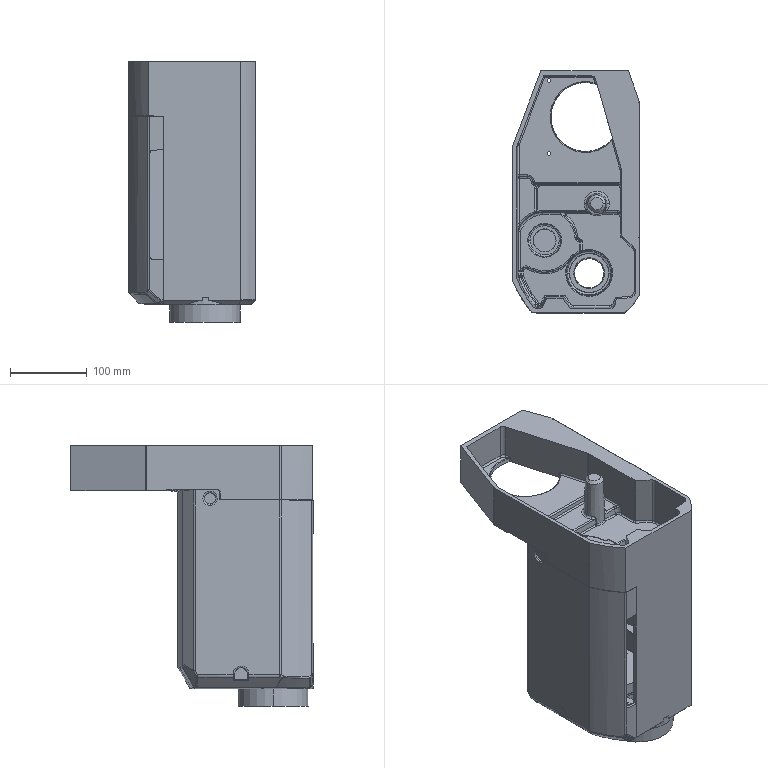Part | SolidWorks | features ICE 11, BaseBody 7, 3DProfileFeature 1, HoleWzd 1 | 1 solid | 941 faces | box 164.786 x 315.34 x 339.5 mm | volume 2454069 mm3 | spline 361 | cylinder 335 | plane 223 | cone 22 | commonest cylinder face diameters 4 x100 2 x50 10 x49 6 x45 12 x36 8 x13